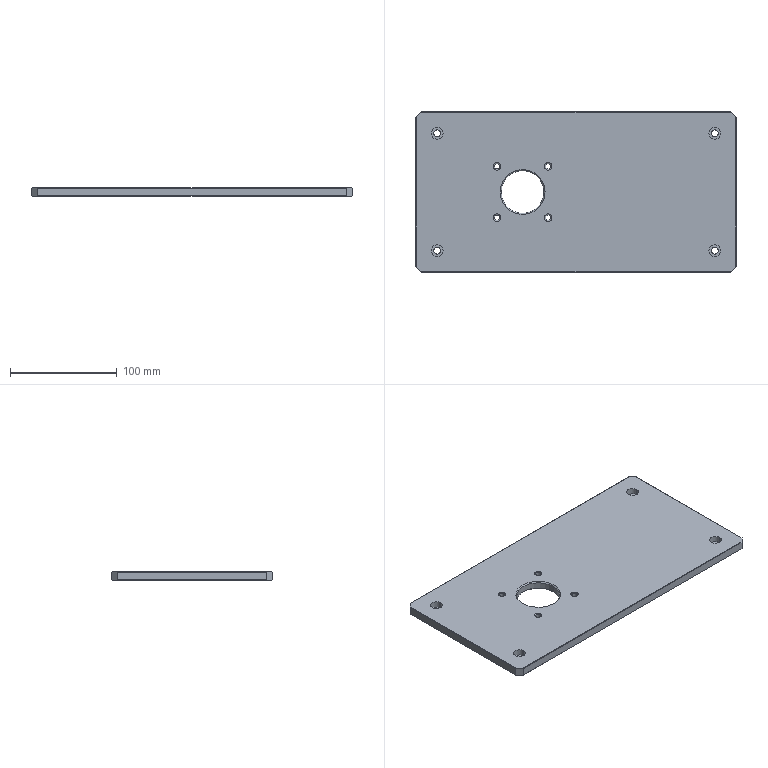Part | NX | 1 solid | 60 faces | box 300 x 150 x 8 mm | volume 346157 mm3 | cylinder 26 | plane 22 | cone 12 | commonest cylinder face diameters 5 x8 6.4 x8 11 x8 40 x2